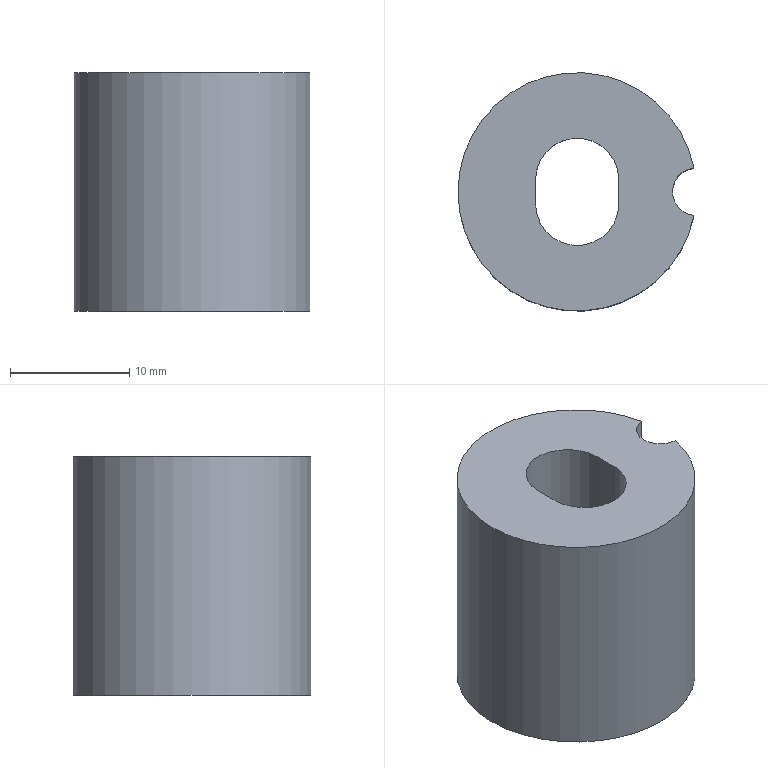Part | NX | features solid 2 | 1 solid | 10 faces | box 19.8 x 20 x 20 mm | volume 4247 mm3 | cylinder 5 | plane 5 | commonest cylinder face diameters 7 x2 4 x1 12.6 x1 20 x1
STEP:
#1=CARTESIAN_POINT('',(-577.966,-395.954,10.8));
#2=VERTEX_POINT('',#1);
#3=CARTESIAN_POINT('',(-577.966,-395.954,30.8));
#4=VERTEX_POINT('',#3);
#5=CARTESIAN_POINT('',(-577.966,-395.954,20.8));
#6=DIRECTION('',(0.,0.,1.));
#7=VECTOR('',#6,1000.);
#8=LINE('',#5,#7);
#9=EDGE_CURVE('',#2,#4,#8,.T.);
#10=ORIENTED_EDGE('',*,*,#9,.T.);
#11=CARTESIAN_POINT('',(-577.966,-391.974,30.8));
#12=VERTEX_POINT('',#11);
#13=CARTESIAN_POINT('',(-587.766,-393.964,30.8));
#14=DIRECTION('',(0.,0.,-1.));
#15=DIRECTION('',(1.,0.,0.));
#16=AXIS2_PLACEMENT_3D('',#13,#14,#15);
#17=CIRCLE('',#16,10.);
#18=EDGE_CURVE('',#4,#12,#17,.T.);
#19=ORIENTED_EDGE('',*,*,#18,.T.);
#20=CARTESIAN_POINT('',(-577.966,-391.974,10.8));
#21=VERTEX_POINT('',#20);
#22=CARTESIAN_POINT('',(-577.966,-391.974,20.8));
#23=DIRECTION('',(0.,0.,1.));
#24=VECTOR('',#23,1000.);
#25=LINE('',#22,#24);
#26=EDGE_CURVE('',#12,#21,#25,.F.);
#27=ORIENTED_EDGE('',*,*,#26,.T.);
#28=CARTESIAN_POINT('',(-587.766,-393.964,10.8));
#29=DIRECTION('',(0.,0.,1.));
#30=DIRECTION('',(1.,0.,0.));
#31=AXIS2_PLACEMENT_3D('',#28,#29,#30);
#32=CIRCLE('',#31,10.);
#33=EDGE_CURVE('',#2,#21,#32,.F.);
#34=ORIENTED_EDGE('',*,*,#33,.F.);
#35=EDGE_LOOP('',(#10,#19,#27,#34));
#36=FACE_BOUND('',#35,.T.);
#37=CARTESIAN_POINT('',(-587.766,-393.964,10.8));
#38=DIRECTION('',(0.,0.,1.));
#39=DIRECTION('',(1.,0.,0.));
#40=AXIS2_PLACEMENT_3D('',#37,#38,#39);
#41=CYLINDRICAL_SURFACE('',#40,10.);
#42=ADVANCED_FACE('',(#36),#41,.T.);
#43=CARTESIAN_POINT('',(-581.466,-393.964,10.8));
#44=VERTEX_POINT('',#43);
#45=CARTESIAN_POINT('',(-587.766,-393.964,10.8));
#46=DIRECTION('',(0.,0.,1.));
#47=DIRECTION('',(1.,0.,0.));
#48=AXIS2_PLACEMENT_3D('',#45,#46,#47);
#49=CIRCLE('',#48,6.3);
#50=EDGE_CURVE('',#44,#44,#49,.F.);
#51=ORIENTED_EDGE('',*,*,#50,.F.);
#52=EDGE_LOOP('',(#51));
#53=FACE_BOUND('',#52,.T.);
#54=ORIENTED_EDGE('',*,*,#33,.T.);
#55=CARTESIAN_POINT('',(-577.766,-393.964,10.8));
#56=DIRECTION('',(0.,0.,1.));
#57=DIRECTION('',(1.,0.,0.));
#58=AXIS2_PLACEMENT_3D('',#55,#56,#57);
#59=CIRCLE('',#58,2.);
#60=EDGE_CURVE('',#2,#21,#59,.F.);
#61=ORIENTED_EDGE('',*,*,#60,.F.);
#62=EDGE_LOOP('',(#54,#61));
#63=FACE_BOUND('',#62,.T.);
#64=CARTESIAN_POINT('',(-587.766,-393.964,10.8));
#65=DIRECTION('',(0.,0.,1.));
#66=DIRECTION('',(1.,0.,0.));
#67=AXIS2_PLACEMENT_3D('',#64,#65,#66);
#68=PLANE('',#67);
#69=ADVANCED_FACE('',(#53,#63),#68,.F.);
#70=CARTESIAN_POINT('',(-591.266,-394.964,30.8));
#71=VERTEX_POINT('',#70);
#72=CARTESIAN_POINT('',(-591.266,-392.964,30.8));
#73=VERTEX_POINT('',#72);
#74=CARTESIAN_POINT('',(-591.266,-394.964,30.8));
#75=DIRECTION('',(0.,1.,0.));
#76=VECTOR('',#75,1000.);
#77=LINE('',#74,#76);
#78=EDGE_CURVE('',#71,#73,#77,.T.);
#79=ORIENTED_EDGE('',*,*,#78,.T.);
#80=CARTESIAN_POINT('',(-584.266,-392.964,30.8));
#81=VERTEX_POINT('',#80);
#82=CARTESIAN_POINT('',(-587.766,-392.964,30.8));
#83=DIRECTION('',(0.,0.,-1.));
#84=DIRECTION('',(1.,0.,0.));
#85=AXIS2_PLACEMENT_3D('',#82,#83,#84);
#86=CIRCLE('',#85,3.5);
#87=EDGE_CURVE('',#73,#81,#86,.T.);
#88=ORIENTED_EDGE('',*,*,#87,.T.);
#89=CARTESIAN_POINT('',(-584.266,-394.964,30.8));
#90=VERTEX_POINT('',#89);
#91=CARTESIAN_POINT('',(-584.266,-394.964,30.8));
#92=DIRECTION('',(0.,1.,0.));
#93=VECTOR('',#92,1000.);
#94=LINE('',#91,#93);
#95=EDGE_CURVE('',#90,#81,#94,.T.);
#96=ORIENTED_EDGE('',*,*,#95,.F.);
#97=CARTESIAN_POINT('',(-587.766,-394.964,30.8));
#98=DIRECTION('',(0.,0.,-1.));
#99=DIRECTION('',(1.,0.,0.));
#100=AXIS2_PLACEMENT_3D('',#97,#98,#99);
#101=CIRCLE('',#100,3.5);
#102=EDGE_CURVE('',#90,#71,#101,.T.);
#103=ORIENTED_EDGE('',*,*,#102,.T.);
#104=EDGE_LOOP('',(#79,#88,#96,#103));
#105=FACE_BOUND('',#104,.T.);
#106=CARTESIAN_POINT('',(-577.766,-393.964,30.8));
#107=DIRECTION('',(0.,0.,-1.));
#108=DIRECTION('',(1.,0.,0.));
#109=AXIS2_PLACEMENT_3D('',#106,#107,#108);
#110=CIRCLE('',#109,2.);
#111=EDGE_CURVE('',#4,#12,#110,.T.);
#112=ORIENTED_EDGE('',*,*,#111,.T.);
#113=ORIENTED_EDGE('',*,*,#18,.F.);
#114=EDGE_LOOP('',(#112,#113));
#115=FACE_BOUND('',#114,.T.);
#116=CARTESIAN_POINT('',(-587.766,-393.964,30.8));
#117=DIRECTION('',(0.,0.,1.));
#118=DIRECTION('',(1.,0.,0.));
#119=AXIS2_PLACEMENT_3D('',#116,#117,#118);
#120=PLANE('',#119);
#121=ADVANCED_FACE('',(#105,#115),#120,.T.);
#122=ORIENTED_EDGE('',*,*,#50,.T.);
#123=EDGE_LOOP('',(#122));
#124=FACE_BOUND('',#123,.T.);
#125=CARTESIAN_POINT('',(-581.466,-393.964,22.8));
#126=VERTEX_POINT('',#125);
#127=CARTESIAN_POINT('',(-587.766,-393.964,22.8));
#128=DIRECTION('',(0.,0.,-1.));
#129=DIRECTION('',(1.,0.,0.));
#130=AXIS2_PLACEMENT_3D('',#127,#128,#129);
#131=CIRCLE('',#130,6.3);
#132=EDGE_CURVE('',#126,#126,#131,.T.);
#133=ORIENTED_EDGE('',*,*,#132,.F.);
#134=EDGE_LOOP('',(#133));
#135=FACE_BOUND('',#134,.T.);
#136=CARTESIAN_POINT('',(-587.766,-393.964,10.8));
#137=DIRECTION('',(0.,0.,1.));
#138=DIRECTION('',(1.,0.,0.));
#139=AXIS2_PLACEMENT_3D('',#136,#137,#138);
#140=CYLINDRICAL_SURFACE('',#139,6.3);
#141=ADVANCED_FACE('',(#124,#135),#140,.F.);
#142=CARTESIAN_POINT('',(-584.266,-394.964,22.8));
#143=VERTEX_POINT('',#142);
#144=CARTESIAN_POINT('',(-591.266,-394.964,22.8));
#145=VERTEX_POINT('',#144);
#146=CARTESIAN_POINT('',(-587.766,-394.964,22.8));
#147=DIRECTION('',(0.,0.,-1.));
#148=DIRECTION('',(1.,0.,0.));
#149=AXIS2_PLACEMENT_3D('',#146,#147,#148);
#150=CIRCLE('',#149,3.5);
#151=EDGE_CURVE('',#143,#145,#150,.T.);
#152=ORIENTED_EDGE('',*,*,#151,.F.);
#153=CARTESIAN_POINT('',(-584.266,-392.964,22.8));
#154=VERTEX_POINT('',#153);
#155=CARTESIAN_POINT('',(-584.266,-393.964,22.8));
#156=DIRECTION('',(0.,1.,0.));
#157=VECTOR('',#156,1000.);
#158=LINE('',#155,#157);
#159=EDGE_CURVE('',#143,#154,#158,.T.);
#160=ORIENTED_EDGE('',*,*,#159,.T.);
#161=CARTESIAN_POINT('',(-591.266,-392.964,22.8));
#162=VERTEX_POINT('',#161);
#163=CARTESIAN_POINT('',(-587.766,-392.964,22.8));
#164=DIRECTION('',(0.,0.,-1.));
#165=DIRECTION('',(1.,0.,0.));
#166=AXIS2_PLACEMENT_3D('',#163,#164,#165);
#167=CIRCLE('',#166,3.5);
#168=EDGE_CURVE('',#162,#154,#167,.T.);
#169=ORIENTED_EDGE('',*,*,#168,.F.);
#170=CARTESIAN_POINT('',(-591.266,-393.964,22.8));
#171=DIRECTION('',(0.,1.,0.));
#172=VECTOR('',#171,1000.);
#173=LINE('',#170,#172);
#174=EDGE_CURVE('',#145,#162,#173,.T.);
#175=ORIENTED_EDGE('',*,*,#174,.F.);
#176=EDGE_LOOP('',(#152,#160,#169,#175));
#177=FACE_BOUND('',#176,.T.);
#178=ORIENTED_EDGE('',*,*,#132,.T.);
#179=EDGE_LOOP('',(#178));
#180=FACE_BOUND('',#179,.T.);
#181=CARTESIAN_POINT('',(-587.766,-393.964,22.8));
#182=DIRECTION('',(0.,0.,1.));
#183=DIRECTION('',(1.,0.,0.));
#184=AXIS2_PLACEMENT_3D('',#181,#182,#183);
#185=PLANE('',#184);
#186=ADVANCED_FACE('',(#177,#180),#185,.F.);
#187=ORIENTED_EDGE('',*,*,#9,.F.);
#188=ORIENTED_EDGE('',*,*,#60,.T.);
#189=ORIENTED_EDGE('',*,*,#26,.F.);
#190=ORIENTED_EDGE('',*,*,#111,.F.);
#191=EDGE_LOOP('',(#187,#188,#189,#190));
#192=FACE_BOUND('',#191,.T.);
#193=CARTESIAN_POINT('',(-577.766,-393.964,10.8));
#194=DIRECTION('',(0.,0.,1.));
#195=DIRECTION('',(1.,0.,0.));
#196=AXIS2_PLACEMENT_3D('',#193,#194,#195);
#197=CYLINDRICAL_SURFACE('',#196,2.);
#198=ADVANCED_FACE('',(#192),#197,.F.);
#199=CARTESIAN_POINT('',(-591.266,-394.964,10.8));
#200=DIRECTION('',(0.,0.,1.));
#201=VECTOR('',#200,1000.);
#202=LINE('',#199,#201);
#203=EDGE_CURVE('',#145,#71,#202,.T.);
#204=ORIENTED_EDGE('',*,*,#203,.F.);
#205=ORIENTED_EDGE('',*,*,#174,.T.);
#206=CARTESIAN_POINT('',(-591.266,-392.964,10.8));
#207=DIRECTION('',(0.,0.,1.));
#208=VECTOR('',#207,1000.);
#209=LINE('',#206,#208);
#210=EDGE_CURVE('',#162,#73,#209,.T.);
#211=ORIENTED_EDGE('',*,*,#210,.T.);
#212=ORIENTED_EDGE('',*,*,#78,.F.);
#213=EDGE_LOOP('',(#204,#205,#211,#212));
#214=FACE_BOUND('',#213,.T.);
#215=CARTESIAN_POINT('',(-591.266,-394.964,10.8));
#216=DIRECTION('',(-1.,0.,0.));
#217=DIRECTION('',(0.,0.,1.));
#218=AXIS2_PLACEMENT_3D('',#215,#216,#217);
#219=PLANE('',#218);
#220=ADVANCED_FACE('',(#214),#219,.F.);
#221=ORIENTED_EDGE('',*,*,#210,.F.);
#222=ORIENTED_EDGE('',*,*,#168,.T.);
#223=CARTESIAN_POINT('',(-584.266,-392.964,10.8));
#224=DIRECTION('',(0.,0.,1.));
#225=VECTOR('',#224,1000.);
#226=LINE('',#223,#225);
#227=EDGE_CURVE('',#154,#81,#226,.T.);
#228=ORIENTED_EDGE('',*,*,#227,.T.);
#229=ORIENTED_EDGE('',*,*,#87,.F.);
#230=EDGE_LOOP('',(#221,#222,#228,#229));
#231=FACE_BOUND('',#230,.T.);
#232=CARTESIAN_POINT('',(-587.766,-392.964,10.8));
#233=DIRECTION('',(0.,0.,1.));
#234=DIRECTION('',(1.,0.,0.));
#235=AXIS2_PLACEMENT_3D('',#232,#233,#234);
#236=CYLINDRICAL_SURFACE('',#235,3.5);
#237=ADVANCED_FACE('',(#231),#236,.F.);
#238=ORIENTED_EDGE('',*,*,#159,.F.);
#239=CARTESIAN_POINT('',(-584.266,-394.964,10.8));
#240=DIRECTION('',(0.,0.,1.));
#241=VECTOR('',#240,1000.);
#242=LINE('',#239,#241);
#243=EDGE_CURVE('',#143,#90,#242,.T.);
#244=ORIENTED_EDGE('',*,*,#243,.T.);
#245=ORIENTED_EDGE('',*,*,#95,.T.);
#246=ORIENTED_EDGE('',*,*,#227,.F.);
#247=EDGE_LOOP('',(#238,#244,#245,#246));
#248=FACE_BOUND('',#247,.T.);
#249=CARTESIAN_POINT('',(-584.266,-394.964,10.8));
#250=DIRECTION('',(-1.,0.,0.));
#251=DIRECTION('',(0.,0.,1.));
#252=AXIS2_PLACEMENT_3D('',#249,#250,#251);
#253=PLANE('',#252);
#254=ADVANCED_FACE('',(#248),#253,.T.);
#255=ORIENTED_EDGE('',*,*,#243,.F.);
#256=ORIENTED_EDGE('',*,*,#151,.T.);
#257=ORIENTED_EDGE('',*,*,#203,.T.);
#258=ORIENTED_EDGE('',*,*,#102,.F.);
#259=EDGE_LOOP('',(#255,#256,#257,#258));
#260=FACE_BOUND('',#259,.T.);
#261=CARTESIAN_POINT('',(-587.766,-394.964,10.8));
#262=DIRECTION('',(0.,0.,1.));
#263=DIRECTION('',(1.,0.,0.));
#264=AXIS2_PLACEMENT_3D('',#261,#262,#263);
#265=CYLINDRICAL_SURFACE('',#264,3.5);
#266=ADVANCED_FACE('',(#260),#265,.F.);
#267=CLOSED_SHELL('',(#42,#69,#121,#141,#186,#198,#220,#237,#254,#266));
#268=MANIFOLD_SOLID_BREP('',#267);
#269=(LENGTH_UNIT()NAMED_UNIT(*)SI_UNIT(.MILLI.,.METRE.));
#270=UNCERTAINTY_MEASURE_WITH_UNIT(LENGTH_MEASURE(0.00001),#269,'','');
#271=(NAMED_UNIT(*)PLANE_ANGLE_UNIT()SI_UNIT($,.RADIAN.));
#272=(NAMED_UNIT(*)SI_UNIT($,.STERADIAN.)SOLID_ANGLE_UNIT());
#273=(GEOMETRIC_REPRESENTATION_CONTEXT(3)GLOBAL_UNCERTAINTY_ASSIGNED_CONTEXT((#270))GLOBAL_UNIT_ASSIGNED_CONTEXT((#269,#271,#272))REPRESENTATION_CONTEXT('',''));
#274=ADVANCED_BREP_SHAPE_REPRESENTATION('',(#268),#273);